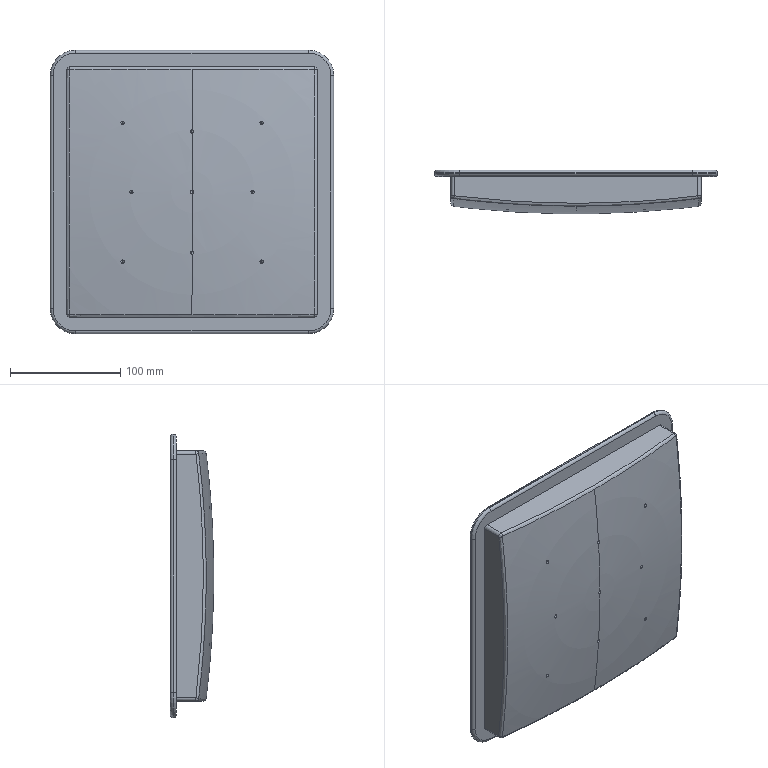Part | SolidWorks | features ICE 6, Fillet 2, RevCut 2, 3DProfileFeature 1, Extrusion 1, Rib 1, Shell 1, SketchPattern 1 | 1 solid | 295 faces | box 257 x 39.299 x 257 mm | volume 199680 mm3 | cylinder 103 | plane 98 | sphere 36 | torus 30 | spline 28 | commonest cylinder face diameters 7.5 x27 2.5 x24 3.3 x8 5 x8 7.3 x8 2 x4